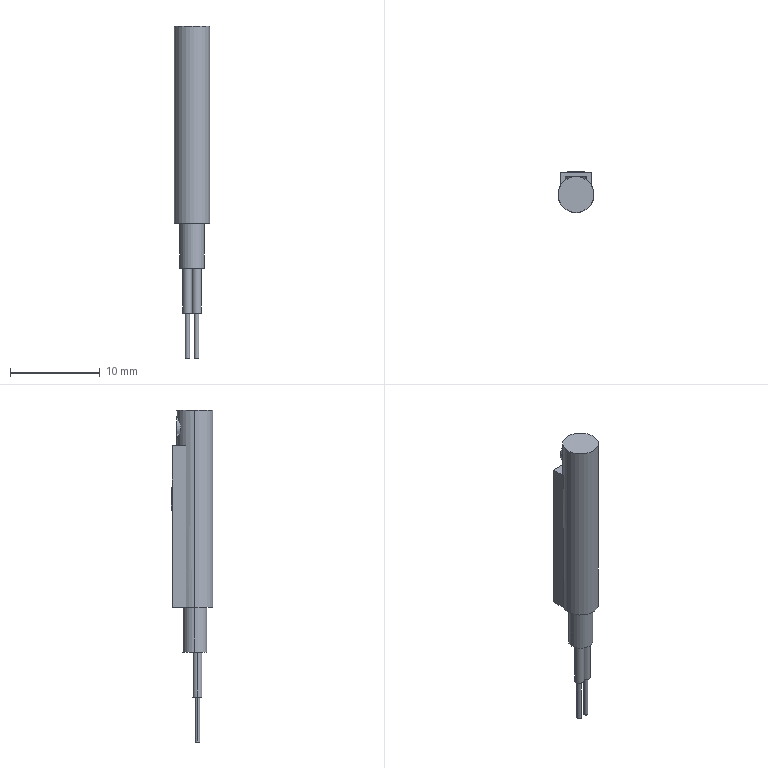Part | NX | 1 solid | 38 faces | box 4 x 4.6 x 37 mm | volume 364.626 mm3 | plane 21 | cylinder 17 | commonest cylinder face diameters 0.5 x4 1 x4 2.4 x3 2.5 x2 2.7 x2 4 x2
STEP:
#1=CARTESIAN_POINT('',(0.,2.,-3.2));
#2=VERTEX_POINT('',#1);
#3=CARTESIAN_POINT('',(0.,1.,-3.2));
#4=VERTEX_POINT('',#3);
#5=CARTESIAN_POINT('',(0.,2.,-3.2));
#6=DIRECTION('',(0.,-1.,0.));
#7=VECTOR('',#6,1000.);
#8=LINE('',#5,#7);
#9=EDGE_CURVE('',#2,#4,#8,.T.);
#10=ORIENTED_EDGE('',*,*,#9,.F.);
#11=CARTESIAN_POINT('',(1.007,2.,-1.347));
#12=VERTEX_POINT('',#11);
#13=CARTESIAN_POINT('',(0.,2.,-2.));
#14=DIRECTION('',(0.,1.,0.));
#15=DIRECTION('',(0.,0.,1.));
#16=AXIS2_PLACEMENT_3D('',#13,#14,#15);
#17=CIRCLE('',#16,1.2);
#18=EDGE_CURVE('',#12,#2,#17,.T.);
#19=ORIENTED_EDGE('',*,*,#18,.F.);
#20=CARTESIAN_POINT('',(1.007,1.,-1.347));
#21=VERTEX_POINT('',#20);
#22=CARTESIAN_POINT('',(1.007,1.,-1.347));
#23=DIRECTION('',(0.,1.,0.));
#24=VECTOR('',#23,1000.);
#25=LINE('',#22,#24);
#26=EDGE_CURVE('',#21,#12,#25,.T.);
#27=ORIENTED_EDGE('',*,*,#26,.F.);
#28=CARTESIAN_POINT('',(0.,1.,-2.));
#29=DIRECTION('',(0.,1.,0.));
#30=DIRECTION('',(0.,0.,1.));
#31=AXIS2_PLACEMENT_3D('',#28,#29,#30);
#32=CIRCLE('',#31,1.2);
#33=EDGE_CURVE('',#21,#4,#32,.T.);
#34=ORIENTED_EDGE('',*,*,#33,.T.);
#35=EDGE_LOOP('',(#10,#19,#27,#34));
#36=FACE_BOUND('',#35,.T.);
#37=CARTESIAN_POINT('',(0.,2.,-2.));
#38=DIRECTION('',(0.,-1.,0.));
#39=DIRECTION('',(0.,0.,-1.));
#40=AXIS2_PLACEMENT_3D('',#37,#38,#39);
#41=CYLINDRICAL_SURFACE('',#40,1.2);
#42=ADVANCED_FACE('',(#36),#41,.T.);
#43=CARTESIAN_POINT('',(0.,2.,-0.75));
#44=VERTEX_POINT('',#43);
#45=CARTESIAN_POINT('',(0.,2.,-3.25));
#46=VERTEX_POINT('',#45);
#47=CARTESIAN_POINT('',(0.,2.,-0.75));
#48=CARTESIAN_POINT('',(0.02817,2.,-0.75));
#49=CARTESIAN_POINT('',(0.05639,1.999,-0.751));
#50=CARTESIAN_POINT('',(0.08452,1.998,-0.7529));
#51=CARTESIAN_POINT('',(0.1126,1.997,-0.7548));
#52=CARTESIAN_POINT('',(0.1407,1.995,-0.7576));
#53=CARTESIAN_POINT('',(0.1685,1.993,-0.7614));
#54=CARTESIAN_POINT('',(0.1824,1.992,-0.7633));
#55=CARTESIAN_POINT('',(0.1963,1.99,-0.7654));
#56=CARTESIAN_POINT('',(0.2101,1.989,-0.7678));
#57=CARTESIAN_POINT('',(0.2238,1.987,-0.7701));
#58=CARTESIAN_POINT('',(0.2376,1.986,-0.7727));
#59=CARTESIAN_POINT('',(0.2513,1.984,-0.7755));
#60=CARTESIAN_POINT('',(0.2787,1.981,-0.7811));
#61=CARTESIAN_POINT('',(0.3059,1.977,-0.7877));
#62=CARTESIAN_POINT('',(0.3327,1.972,-0.7951));
#63=CARTESIAN_POINT('',(0.3596,1.968,-0.8025));
#64=CARTESIAN_POINT('',(0.3861,1.963,-0.8108));
#65=CARTESIAN_POINT('',(0.4122,1.957,-0.8199));
#66=CARTESIAN_POINT('',(0.4383,1.952,-0.829));
#67=CARTESIAN_POINT('',(0.464,1.946,-0.839));
#68=CARTESIAN_POINT('',(0.4892,1.939,-0.8497));
#69=CARTESIAN_POINT('',(0.5144,1.933,-0.8604));
#70=CARTESIAN_POINT('',(0.5393,1.926,-0.872));
#71=CARTESIAN_POINT('',(0.5637,1.919,-0.8843));
#72=CARTESIAN_POINT('',(0.5881,1.912,-0.8966));
#73=CARTESIAN_POINT('',(0.612,1.904,-0.9097));
#74=CARTESIAN_POINT('',(0.6354,1.896,-0.9235));
#75=CARTESIAN_POINT('',(0.6588,1.889,-0.9373));
#76=CARTESIAN_POINT('',(0.6817,1.88,-0.9519));
#77=CARTESIAN_POINT('',(0.704,1.872,-0.9671));
#78=CARTESIAN_POINT('',(0.7263,1.864,-0.9823));
#79=CARTESIAN_POINT('',(0.748,1.855,-0.9981));
#80=CARTESIAN_POINT('',(0.7691,1.846,-1.015));
#81=CARTESIAN_POINT('',(0.7901,1.837,-1.031));
#82=CARTESIAN_POINT('',(0.8106,1.828,-1.048));
#83=CARTESIAN_POINT('',(0.8306,1.819,-1.066));
#84=CARTESIAN_POINT('',(0.8506,1.81,-1.084));
#85=CARTESIAN_POINT('',(0.87,1.801,-1.102));
#86=CARTESIAN_POINT('',(0.8888,1.792,-1.121));
#87=CARTESIAN_POINT('',(0.9076,1.782,-1.14));
#88=CARTESIAN_POINT('',(0.9258,1.773,-1.16));
#89=CARTESIAN_POINT('',(0.9434,1.764,-1.18));
#90=CARTESIAN_POINT('',(0.961,1.754,-1.2));
#91=CARTESIAN_POINT('',(0.9779,1.745,-1.221));
#92=CARTESIAN_POINT('',(0.9942,1.735,-1.242));
#93=CARTESIAN_POINT('',(1.01,1.726,-1.264));
#94=CARTESIAN_POINT('',(1.026,1.717,-1.285));
#95=CARTESIAN_POINT('',(1.041,1.708,-1.308));
#96=CARTESIAN_POINT('',(1.056,1.699,-1.33));
#97=CARTESIAN_POINT('',(1.07,1.69,-1.353));
#98=CARTESIAN_POINT('',(1.083,1.681,-1.376));
#99=CARTESIAN_POINT('',(1.09,1.677,-1.388));
#100=CARTESIAN_POINT('',(1.096,1.673,-1.399));
#101=CARTESIAN_POINT('',(1.102,1.669,-1.411));
#102=CARTESIAN_POINT('',(1.109,1.665,-1.422));
#103=CARTESIAN_POINT('',(1.115,1.661,-1.434));
#104=CARTESIAN_POINT('',(1.121,1.657,-1.446));
#105=CARTESIAN_POINT('',(1.132,1.649,-1.47));
#106=CARTESIAN_POINT('',(1.143,1.641,-1.494));
#107=CARTESIAN_POINT('',(1.154,1.634,-1.519));
#108=CARTESIAN_POINT('',(1.164,1.626,-1.544));
#109=CARTESIAN_POINT('',(1.174,1.619,-1.569));
#110=CARTESIAN_POINT('',(1.182,1.613,-1.595));
#111=CARTESIAN_POINT('',(1.191,1.607,-1.62));
#112=CARTESIAN_POINT('',(1.199,1.601,-1.646));
#113=CARTESIAN_POINT('',(1.206,1.595,-1.673));
#114=CARTESIAN_POINT('',(1.214,1.59,-1.699));
#115=CARTESIAN_POINT('',(1.22,1.585,-1.726));
#116=CARTESIAN_POINT('',(1.225,1.581,-1.753));
#117=CARTESIAN_POINT('',(1.231,1.577,-1.779));
#118=CARTESIAN_POINT('',(1.235,1.573,-1.806));
#119=CARTESIAN_POINT('',(1.239,1.57,-1.834));
#120=CARTESIAN_POINT('',(1.243,1.567,-1.861));
#121=CARTESIAN_POINT('',(1.245,1.565,-1.888));
#122=CARTESIAN_POINT('',(1.247,1.563,-1.916));
#123=CARTESIAN_POINT('',(1.248,1.563,-1.93));
#124=CARTESIAN_POINT('',(1.249,1.562,-1.944));
#125=CARTESIAN_POINT('',(1.249,1.562,-1.958));
#126=CARTESIAN_POINT('',(1.25,1.561,-1.972));
#127=CARTESIAN_POINT('',(1.25,1.561,-1.986));
#128=CARTESIAN_POINT('',(1.25,1.561,-2.));
#129=CARTESIAN_POINT('',(1.25,1.561,-2.014));
#130=CARTESIAN_POINT('',(1.25,1.561,-2.028));
#131=CARTESIAN_POINT('',(1.249,1.562,-2.042));
#132=CARTESIAN_POINT('',(1.249,1.562,-2.055));
#133=CARTESIAN_POINT('',(1.248,1.563,-2.069));
#134=CARTESIAN_POINT('',(1.247,1.563,-2.083));
#135=CARTESIAN_POINT('',(1.245,1.565,-2.111));
#136=CARTESIAN_POINT('',(1.243,1.567,-2.139));
#137=CARTESIAN_POINT('',(1.239,1.57,-2.166));
#138=CARTESIAN_POINT('',(1.237,1.571,-2.18));
#139=CARTESIAN_POINT('',(1.235,1.573,-2.193));
#140=CARTESIAN_POINT('',(1.233,1.575,-2.207));
#141=CARTESIAN_POINT('',(1.231,1.577,-2.22));
#142=CARTESIAN_POINT('',(1.228,1.579,-2.234));
#143=CARTESIAN_POINT('',(1.225,1.581,-2.247));
#144=CARTESIAN_POINT('',(1.22,1.585,-2.274));
#145=CARTESIAN_POINT('',(1.214,1.59,-2.3));
#146=CARTESIAN_POINT('',(1.207,1.595,-2.327));
#147=CARTESIAN_POINT('',(1.199,1.6,-2.353));
#148=CARTESIAN_POINT('',(1.191,1.606,-2.379));
#149=CARTESIAN_POINT('',(1.183,1.613,-2.405));
#150=CARTESIAN_POINT('',(1.174,1.619,-2.43));
#151=CARTESIAN_POINT('',(1.164,1.626,-2.456));
#152=CARTESIAN_POINT('',(1.154,1.633,-2.48));
#153=CARTESIAN_POINT('',(1.144,1.641,-2.505));
#154=CARTESIAN_POINT('',(1.133,1.648,-2.529));
#155=CARTESIAN_POINT('',(1.121,1.656,-2.553));
#156=CARTESIAN_POINT('',(1.115,1.66,-2.565));
#157=CARTESIAN_POINT('',(1.109,1.664,-2.577));
#158=CARTESIAN_POINT('',(1.103,1.668,-2.589));
#159=CARTESIAN_POINT('',(1.097,1.673,-2.6));
#160=CARTESIAN_POINT('',(1.09,1.677,-2.612));
#161=CARTESIAN_POINT('',(1.084,1.681,-2.623));
#162=CARTESIAN_POINT('',(1.07,1.69,-2.646));
#163=CARTESIAN_POINT('',(1.056,1.699,-2.669));
#164=CARTESIAN_POINT('',(1.041,1.708,-2.692));
#165=CARTESIAN_POINT('',(1.026,1.717,-2.714));
#166=CARTESIAN_POINT('',(1.011,1.726,-2.736));
#167=CARTESIAN_POINT('',(0.9946,1.735,-2.757));
#168=CARTESIAN_POINT('',(0.9784,1.744,-2.778));
#169=CARTESIAN_POINT('',(0.9615,1.754,-2.799));
#170=CARTESIAN_POINT('',(0.9439,1.763,-2.819));
#171=CARTESIAN_POINT('',(0.9264,1.773,-2.84));
#172=CARTESIAN_POINT('',(0.9082,1.782,-2.859));
#173=CARTESIAN_POINT('',(0.8894,1.791,-2.878));
#174=CARTESIAN_POINT('',(0.8706,1.801,-2.897));
#175=CARTESIAN_POINT('',(0.8512,1.81,-2.916));
#176=CARTESIAN_POINT('',(0.8313,1.819,-2.933));
#177=CARTESIAN_POINT('',(0.8213,1.824,-2.942));
#178=CARTESIAN_POINT('',(0.8112,1.828,-2.951));
#179=CARTESIAN_POINT('',(0.801,1.833,-2.96));
#180=CARTESIAN_POINT('',(0.7908,1.837,-2.968));
#181=CARTESIAN_POINT('',(0.7804,1.842,-2.977));
#182=CARTESIAN_POINT('',(0.7698,1.846,-2.985));
#183=CARTESIAN_POINT('',(0.7487,1.855,-3.001));
#184=CARTESIAN_POINT('',(0.727,1.863,-3.017));
#185=CARTESIAN_POINT('',(0.7046,1.872,-3.032));
#186=CARTESIAN_POINT('',(0.6823,1.88,-3.048));
#187=CARTESIAN_POINT('',(0.6594,1.888,-3.062));
#188=CARTESIAN_POINT('',(0.6359,1.896,-3.076));
#189=CARTESIAN_POINT('',(0.6124,1.904,-3.09));
#190=CARTESIAN_POINT('',(0.5885,1.912,-3.103));
#191=CARTESIAN_POINT('',(0.564,1.919,-3.116));
#192=CARTESIAN_POINT('',(0.5395,1.926,-3.128));
#193=CARTESIAN_POINT('',(0.5146,1.933,-3.139));
#194=CARTESIAN_POINT('',(0.4893,1.939,-3.15));
#195=CARTESIAN_POINT('',(0.464,1.946,-3.161));
#196=CARTESIAN_POINT('',(0.4383,1.952,-3.171));
#197=CARTESIAN_POINT('',(0.4122,1.957,-3.18));
#198=CARTESIAN_POINT('',(0.3862,1.963,-3.189));
#199=CARTESIAN_POINT('',(0.3597,1.968,-3.197));
#200=CARTESIAN_POINT('',(0.3328,1.972,-3.205));
#201=CARTESIAN_POINT('',(0.306,1.977,-3.212));
#202=CARTESIAN_POINT('',(0.2788,1.981,-3.219));
#203=CARTESIAN_POINT('',(0.2513,1.984,-3.224));
#204=CARTESIAN_POINT('',(0.2239,1.988,-3.23));
#205=CARTESIAN_POINT('',(0.1962,1.991,-3.235));
#206=CARTESIAN_POINT('',(0.1684,1.993,-3.239));
#207=CARTESIAN_POINT('',(0.1406,1.995,-3.242));
#208=CARTESIAN_POINT('',(0.1127,1.997,-3.245));
#209=CARTESIAN_POINT('',(0.08455,1.998,-3.247));
#210=CARTESIAN_POINT('',(0.05645,1.999,-3.249));
#211=CARTESIAN_POINT('',(0.02822,2.,-3.25));
#212=CARTESIAN_POINT('',(0.,2.,-3.25));
#213=B_SPLINE_CURVE_WITH_KNOTS('',3,(#47,#48,#49,#50,#51,#52,#53,#54,#55,#56,#57,#58,#59,#60,#61,#62,#63,#64,#65,#66,#67,#68,#69,#70,#71,#72,#73,#74,#75,#76,#77,#78,#79,#80,#81,#82,#83,#84,#85,#86,#87,#88,#89,#90,#91,#92,#93,#94,#95,#96,#97,#98,#99,#100,#101,#102,#103,#104,#105,#106,#107,#108,#109,#110,#111,#112,#113,#114,#115,#116,#117,#118,#119,#120,#121,#122,#123,#124,#125,#126,#127,#128,#129,#130,#131,#132,#133,#134,#135,#136,#137,#138,#139,#140,#141,#142,#143,#144,#145,#146,#147,#148,#149,#150,#151,#152,#153,#154,#155,#156,#157,#158,#159,#160,#161,#162,#163,#164,#165,#166,#167,#168,#169,#170,#171,#172,#173,#174,#175,#176,#177,#178,#179,#180,#181,#182,#183,#184,#185,#186,#187,#188,#189,#190,#191,#192,#193,#194,#195,#196,#197,#198,#199,#200,#201,#202,#203,#204,#205,#206,#207,#208,#209,#210,#211,#212),.UNSPECIFIED.,.F.,.F.,(4,3,3,3,3,3,3,3,3,3,3,3,3,3,3,3,3,3,3,3,3,3,3,3,3,3,3,3,3,3,3,3,3,3,3,3,3,3,3,3,3,3,3,3,3,3,3,3,3,3,3,3,3,3,3,4),(0.,0.08461,0.1692,0.2114,0.2537,0.3383,0.4229,0.5074,0.592,0.6768,0.7617,0.8463,0.9308,1.016,1.101,1.186,1.271,1.356,1.397,1.439,1.522,1.606,1.689,1.773,1.856,1.939,1.981,2.022,2.064,2.106,2.189,2.231,2.272,2.356,2.439,2.522,2.606,2.647,2.689,2.774,2.859,2.944,3.029,3.113,3.156,3.198,3.283,3.368,3.453,3.538,3.622,3.707,3.792,3.876,3.961,4.045),.UNSPECIFIED.);
#214=EDGE_CURVE('',#44,#46,#213,.T.);
#215=ORIENTED_EDGE('',*,*,#214,.T.);
#216=CARTESIAN_POINT('',(0.,1.,-3.25));
#217=VERTEX_POINT('',#216);
#218=CARTESIAN_POINT('',(0.,2.6,-3.25));
#219=DIRECTION('',(0.,-1.,0.));
#220=VECTOR('',#219,1000.);
#221=LINE('',#218,#220);
#222=EDGE_CURVE('',#217,#46,#221,.F.);
#223=ORIENTED_EDGE('',*,*,#222,.F.);
#224=CARTESIAN_POINT('',(0.,1.,-0.75));
#225=VERTEX_POINT('',#224);
#226=CARTESIAN_POINT('',(0.,1.,-2.));
#227=DIRECTION('',(0.,1.,0.));
#228=DIRECTION('',(0.,0.,1.));
#229=AXIS2_PLACEMENT_3D('',#226,#227,#228);
#230=CIRCLE('',#229,1.25);
#231=EDGE_CURVE('',#225,#217,#230,.T.);
#232=ORIENTED_EDGE('',*,*,#231,.F.);
#233=CARTESIAN_POINT('',(0.,2.6,-0.75));
#234=DIRECTION('',(0.,-1.,0.));
#235=VECTOR('',#234,1000.);
#236=LINE('',#233,#235);
#237=EDGE_CURVE('',#225,#44,#236,.F.);
#238=ORIENTED_EDGE('',*,*,#237,.T.);
#239=EDGE_LOOP('',(#215,#223,#232,#238));
#240=FACE_BOUND('',#239,.T.);
#241=CARTESIAN_POINT('',(0.,2.6,-2.));
#242=DIRECTION('',(0.,-1.,0.));
#243=DIRECTION('',(0.,0.,-1.));
#244=AXIS2_PLACEMENT_3D('',#241,#242,#243);
#245=CYLINDRICAL_SURFACE('',#244,1.25);
#246=ADVANCED_FACE('',(#240),#245,.F.);
#247=CARTESIAN_POINT('',(-0.7696,-0.3,-32.));
#248=VERTEX_POINT('',#247);
#249=CARTESIAN_POINT('',(-0.2696,-0.3,-32.));
#250=VERTEX_POINT('',#249);
#251=CARTESIAN_POINT('',(-0.5196,-0.3,-32.));
#252=DIRECTION('',(0.,0.,-1.));
#253=DIRECTION('',(1.,0.,0.));
#254=AXIS2_PLACEMENT_3D('',#251,#252,#253);
#255=CIRCLE('',#254,0.25);
#256=EDGE_CURVE('',#248,#250,#255,.T.);
#257=ORIENTED_EDGE('',*,*,#256,.T.);
#258=CARTESIAN_POINT('',(-0.2696,-0.3,-37.));
#259=VERTEX_POINT('',#258);
#260=CARTESIAN_POINT('',(-0.2696,-0.3,-37.));
#261=DIRECTION('',(0.,0.,1.));
#262=VECTOR('',#261,1000.);
#263=LINE('',#260,#262);
#264=EDGE_CURVE('',#259,#250,#263,.T.);
#265=ORIENTED_EDGE('',*,*,#264,.F.);
#266=CARTESIAN_POINT('',(-0.7696,-0.3,-37.));
#267=VERTEX_POINT('',#266);
#268=CARTESIAN_POINT('',(-0.5196,-0.3,-37.));
#269=DIRECTION('',(0.,0.,-1.));
#270=DIRECTION('',(1.,0.,0.));
#271=AXIS2_PLACEMENT_3D('',#268,#269,#270);
#272=CIRCLE('',#271,0.25);
#273=EDGE_CURVE('',#267,#259,#272,.T.);
#274=ORIENTED_EDGE('',*,*,#273,.F.);
#275=CARTESIAN_POINT('',(-0.7696,-0.3,-37.));
#276=DIRECTION('',(0.,0.,1.));
#277=VECTOR('',#276,1000.);
#278=LINE('',#275,#277);
#279=EDGE_CURVE('',#267,#248,#278,.T.);
#280=ORIENTED_EDGE('',*,*,#279,.T.);
#281=EDGE_LOOP('',(#257,#265,#274,#280));
#282=FACE_BOUND('',#281,.T.);
#283=CARTESIAN_POINT('',(-0.5196,-0.3,-37.));
#284=DIRECTION('',(0.,0.,1.));
#285=DIRECTION('',(1.,0.,0.));
#286=AXIS2_PLACEMENT_3D('',#283,#284,#285);
#287=CYLINDRICAL_SURFACE('',#286,0.25);
#288=ADVANCED_FACE('',(#282),#287,.T.);
#289=CARTESIAN_POINT('',(0.7696,-0.3,-32.));
#290=VERTEX_POINT('',#289);
#291=CARTESIAN_POINT('',(0.2696,-0.3,-32.));
#292=VERTEX_POINT('',#291);
#293=CARTESIAN_POINT('',(0.5196,-0.3,-32.));
#294=DIRECTION('',(0.,0.,-1.));
#295=DIRECTION('',(-1.,0.,0.));
#296=AXIS2_PLACEMENT_3D('',#293,#294,#295);
#297=CIRCLE('',#296,0.25);
#298=EDGE_CURVE('',#290,#292,#297,.T.);
#299=ORIENTED_EDGE('',*,*,#298,.T.);
#300=CARTESIAN_POINT('',(0.2696,-0.3,-37.));
#301=VERTEX_POINT('',#300);
#302=CARTESIAN_POINT('',(0.2696,-0.3,-37.));
#303=DIRECTION('',(0.,0.,1.));
#304=VECTOR('',#303,1000.);
#305=LINE('',#302,#304);
#306=EDGE_CURVE('',#292,#301,#305,.F.);
#307=ORIENTED_EDGE('',*,*,#306,.T.);
#308=CARTESIAN_POINT('',(0.7696,-0.3,-37.));
#309=VERTEX_POINT('',#308);
#310=CARTESIAN_POINT('',(0.5196,-0.3,-37.));
#311=DIRECTION('',(0.,0.,-1.));
#312=DIRECTION('',(-1.,0.,0.));
#313=AXIS2_PLACEMENT_3D('',#310,#311,#312);
#314=CIRCLE('',#313,0.25);
#315=EDGE_CURVE('',#309,#301,#314,.T.);
#316=ORIENTED_EDGE('',*,*,#315,.F.);
#317=CARTESIAN_POINT('',(0.7696,-0.3,-37.));
#318=DIRECTION('',(0.,0.,1.));
#319=VECTOR('',#318,1000.);
#320=LINE('',#317,#319);
#321=EDGE_CURVE('',#290,#309,#320,.F.);
#322=ORIENTED_EDGE('',*,*,#321,.F.);
#323=EDGE_LOOP('',(#299,#307,#316,#322));
#324=FACE_BOUND('',#323,.T.);
#325=CARTESIAN_POINT('',(0.5196,-0.3,-37.));
#326=DIRECTION('',(0.,0.,1.));
#327=DIRECTION('',(1.,0.,0.));
#328=AXIS2_PLACEMENT_3D('',#325,#326,#327);
#329=CYLINDRICAL_SURFACE('',#328,0.25);
#330=ADVANCED_FACE('',(#324),#329,.T.);
#331=CARTESIAN_POINT('',(-1.02,-0.3,-27.));
#332=VERTEX_POINT('',#331);
#333=CARTESIAN_POINT('',(-0.01962,-0.3,-27.));
#334=VERTEX_POINT('',#333);
#335=CARTESIAN_POINT('',(-0.5196,-0.3,-27.));
#336=DIRECTION('',(0.,0.,-1.));
#337=DIRECTION('',(-1.,0.,0.));
#338=AXIS2_PLACEMENT_3D('',#335,#336,#337);
#339=CIRCLE('',#338,0.5);
#340=EDGE_CURVE('',#332,#334,#339,.T.);
#341=ORIENTED_EDGE('',*,*,#340,.T.);
#342=CARTESIAN_POINT('',(-0.01962,-0.3,-32.));
#343=VERTEX_POINT('',#342);
#344=CARTESIAN_POINT('',(-0.01962,-0.3,-32.));
#345=DIRECTION('',(0.,0.,1.));
#346=VECTOR('',#345,1000.);
#347=LINE('',#344,#346);
#348=EDGE_CURVE('',#343,#334,#347,.T.);
#349=ORIENTED_EDGE('',*,*,#348,.F.);
#350=CARTESIAN_POINT('',(-1.02,-0.3,-32.));
#351=VERTEX_POINT('',#350);
#352=CARTESIAN_POINT('',(-0.5196,-0.3,-32.));
#353=DIRECTION('',(0.,0.,-1.));
#354=DIRECTION('',(-1.,0.,0.));
#355=AXIS2_PLACEMENT_3D('',#352,#353,#354);
#356=CIRCLE('',#355,0.5);
#357=EDGE_CURVE('',#351,#343,#356,.T.);
#358=ORIENTED_EDGE('',*,*,#357,.F.);
#359=CARTESIAN_POINT('',(-1.02,-0.3,-32.));
#360=DIRECTION('',(0.,0.,1.));
#361=VECTOR('',#360,1000.);
#362=LINE('',#359,#361);
#363=EDGE_CURVE('',#351,#332,#362,.T.);
#364=ORIENTED_EDGE('',*,*,#363,.T.);
#365=EDGE_LOOP('',(#341,#349,#358,#364));
#366=FACE_BOUND('',#365,.T.);
#367=CARTESIAN_POINT('',(-0.5196,-0.3,-32.));
#368=DIRECTION('',(0.,0.,1.));
#369=DIRECTION('',(1.,0.,0.));
#370=AXIS2_PLACEMENT_3D('',#367,#368,#369);
#371=CYLINDRICAL_SURFACE('',#370,0.5);
#372=ADVANCED_FACE('',(#366),#371,.T.);
#373=CARTESIAN_POINT('',(1.02,-0.3,-27.));
#374=VERTEX_POINT('',#373);
#375=CARTESIAN_POINT('',(0.01962,-0.3,-27.));
#376=VERTEX_POINT('',#375);
#377=CARTESIAN_POINT('',(0.5196,-0.3,-27.));
#378=DIRECTION('',(0.,0.,-1.));
#379=DIRECTION('',(-1.,0.,0.));
#380=AXIS2_PLACEMENT_3D('',#377,#378,#379);
#381=CIRCLE('',#380,0.5);
#382=EDGE_CURVE('',#374,#376,#381,.T.);
#383=ORIENTED_EDGE('',*,*,#382,.T.);
#384=CARTESIAN_POINT('',(0.01962,-0.3,-32.));
#385=VERTEX_POINT('',#384);
#386=CARTESIAN_POINT('',(0.01962,-0.3,-32.));
#387=DIRECTION('',(0.,0.,1.));
#388=VECTOR('',#387,1000.);
#389=LINE('',#386,#388);
#390=EDGE_CURVE('',#376,#385,#389,.F.);
#391=ORIENTED_EDGE('',*,*,#390,.T.);
#392=CARTESIAN_POINT('',(1.02,-0.3,-32.));
#393=VERTEX_POINT('',#392);
#394=CARTESIAN_POINT('',(0.5196,-0.3,-32.));
#395=DIRECTION('',(0.,0.,-1.));
#396=DIRECTION('',(-1.,0.,0.));
#397=AXIS2_PLACEMENT_3D('',#394,#395,#396);
#398=CIRCLE('',#397,0.5);
#399=EDGE_CURVE('',#393,#385,#398,.T.);
#400=ORIENTED_EDGE('',*,*,#399,.F.);
#401=CARTESIAN_POINT('',(1.02,-0.3,-32.));
#402=DIRECTION('',(0.,0.,1.));
#403=VECTOR('',#402,1000.);
#404=LINE('',#401,#403);
#405=EDGE_CURVE('',#374,#393,#404,.F.);
#406=ORIENTED_EDGE('',*,*,#405,.F.);
#407=EDGE_LOOP('',(#383,#391,#400,#406));
#408=FACE_BOUND('',#407,.T.);
#409=CARTESIAN_POINT('',(0.5196,-0.3,-32.));
#410=DIRECTION('',(0.,0.,1.));
#411=DIRECTION('',(1.,0.,0.));
#412=AXIS2_PLACEMENT_3D('',#409,#410,#411);
#413=CYLINDRICAL_SURFACE('',#412,0.5);
#414=ADVANCED_FACE('',(#408),#413,.T.);
#415=CARTESIAN_POINT('',(1.35,0.,-27.));
#416=VERTEX_POINT('',#415);
#417=CARTESIAN_POINT('',(-1.35,0.,-27.));
#418=VERTEX_POINT('',#417);
#419=CARTESIAN_POINT('',(0.,0.,-27.));
#420=DIRECTION('',(0.,0.,-1.));
#421=DIRECTION('',(-1.,0.,0.));
#422=AXIS2_PLACEMENT_3D('',#419,#420,#421);
#423=CIRCLE('',#422,1.35);
#424=EDGE_CURVE('',#416,#418,#423,.T.);
#425=ORIENTED_EDGE('',*,*,#424,.F.);
#426=CARTESIAN_POINT('',(1.35,0.,-22.));
#427=VERTEX_POINT('',#426);
#428=CARTESIAN_POINT('',(1.35,0.,-27.));
#429=DIRECTION('',(0.,0.,1.));
#430=VECTOR('',#429,1000.);
#431=LINE('',#428,#430);
#432=EDGE_CURVE('',#416,#427,#431,.T.);
#433=ORIENTED_EDGE('',*,*,#432,.T.);
#434=CARTESIAN_POINT('',(-1.35,0.,-22.));
#435=VERTEX_POINT('',#434);
#436=CARTESIAN_POINT('',(0.,0.,-22.));
#437=DIRECTION('',(0.,0.,-1.));
#438=DIRECTION('',(1.,0.,0.));
#439=AXIS2_PLACEMENT_3D('',#436,#437,#438);
#440=CIRCLE('',#439,1.35);
#441=EDGE_CURVE('',#427,#435,#440,.T.);
#442=ORIENTED_EDGE('',*,*,#441,.T.);
#443=CARTESIAN_POINT('',(-1.35,0.,-27.));
#444=DIRECTION('',(0.,0.,1.));
#445=VECTOR('',#444,1000.);
#446=LINE('',#443,#445);
#447=EDGE_CURVE('',#418,#435,#446,.T.);
#448=ORIENTED_EDGE('',*,*,#447,.F.);
#449=EDGE_LOOP('',(#425,#433,#442,#448));
#450=FACE_BOUND('',#449,.T.);
#451=CARTESIAN_POINT('',(0.,0.,-27.));
#452=DIRECTION('',(0.,0.,1.));
#453=DIRECTION('',(1.,0.,0.));
#454=AXIS2_PLACEMENT_3D('',#451,#452,#453);
#455=CYLINDRICAL_SURFACE('',#454,1.35);
#456=ADVANCED_FACE('',(#450),#455,.T.);
#457=CARTESIAN_POINT('',(-2.,0.,0.));
#458=VERTEX_POINT('',#457);
#459=CARTESIAN_POINT('',(2.,0.,0.));
#460=VERTEX_POINT('',#459);
#461=CARTESIAN_POINT('',(0.,0.,0.));
#462=DIRECTION('',(0.,0.,1.));
#463=DIRECTION('',(1.,0.,0.));
#464=AXIS2_PLACEMENT_3D('',#461,#462,#463);
#465=CIRCLE('',#464,2.);
#466=EDGE_CURVE('',#458,#460,#465,.T.);
#467=ORIENTED_EDGE('',*,*,#466,.F.);
#468=CARTESIAN_POINT('',(-2.,0.,-22.));
#469=VERTEX_POINT('',#468);
#470=CARTESIAN_POINT('',(-2.,0.,-22.));
#471=DIRECTION('',(0.,0.,1.));
#472=VECTOR('',#471,1000.);
#473=LINE('',#470,#472);
#474=EDGE_CURVE('',#458,#469,#473,.F.);
#475=ORIENTED_EDGE('',*,*,#474,.T.);
#476=CARTESIAN_POINT('',(2.,0.,-22.));
#477=VERTEX_POINT('',#476);
#478=CARTESIAN_POINT('',(0.,0.,-22.));
#479=DIRECTION('',(0.,0.,1.));
#480=DIRECTION('',(1.,0.,0.));
#481=AXIS2_PLACEMENT_3D('',#478,#479,#480);
#482=CIRCLE('',#481,2.);
#483=EDGE_CURVE('',#469,#477,#482,.T.);
#484=ORIENTED_EDGE('',*,*,#483,.T.);
#485=CARTESIAN_POINT('',(2.,0.,-22.));
#486=DIRECTION('',(0.,0.,1.));
#487=VECTOR('',#486,1000.);
#488=LINE('',#485,#487);
#489=EDGE_CURVE('',#460,#477,#488,.F.);
#490=ORIENTED_EDGE('',*,*,#489,.F.);
#491=EDGE_LOOP('',(#467,#475,#484,#490));
#492=FACE_BOUND('',#491,.T.);
#493=CARTESIAN_POINT('',(0.,0.,-22.));
#494=DIRECTION('',(0.,0.,1.));
#495=DIRECTION('',(1.,0.,0.));
#496=AXIS2_PLACEMENT_3D('',#493,#494,#495);
#497=CYLINDRICAL_SURFACE('',#496,2.);
#498=ADVANCED_FACE('',(#492),#497,.T.);
#499=CARTESIAN_POINT('',(-1.007,2.,-2.653));
#500=VERTEX_POINT('',#499);
#501=CARTESIAN_POINT('',(0.6531,2.,-0.9933));
#502=VERTEX_POINT('',#501);
#503=CARTESIAN_POINT('',(0.,2.,-2.));
#504=DIRECTION('',(0.,1.,0.));
#505=DIRECTION('',(0.,0.,1.));
#506=AXIS2_PLACEMENT_3D('',#503,#504,#505);
#507=CIRCLE('',#506,1.2);
#508=EDGE_CURVE('',#500,#502,#507,.T.);
#509=ORIENTED_EDGE('',*,*,#508,.F.);
#510=CARTESIAN_POINT('',(-1.007,1.,-2.653));
#511=VERTEX_POINT('',#510);
#512=CARTESIAN_POINT('',(-1.007,1.,-2.653));
#513=DIRECTION('',(0.,1.,0.));
#514=VECTOR('',#513,1000.);
#515=LINE('',#512,#514);
#516=EDGE_CURVE('',#511,#500,#515,.T.);
#517=ORIENTED_EDGE('',*,*,#516,.F.);
#518=CARTESIAN_POINT('',(0.6531,1.,-0.9933));
#519=VERTEX_POINT('',#518);
#520=CARTESIAN_POINT('',(0.,1.,-2.));
#521=DIRECTION('',(0.,1.,0.));
#522=DIRECTION('',(0.,0.,1.));
#523=AXIS2_PLACEMENT_3D('',#520,#521,#522);
#524=CIRCLE('',#523,1.2);
#525=EDGE_CURVE('',#511,#519,#524,.T.);
#526=ORIENTED_EDGE('',*,*,#525,.T.);
#527=CARTESIAN_POINT('',(0.6531,1.,-0.9933));
#528=DIRECTION('',(0.,1.,0.));
#529=VECTOR('',#528,1000.);
#530=LINE('',#527,#529);
#531=EDGE_CURVE('',#519,#502,#530,.T.);
#532=ORIENTED_EDGE('',*,*,#531,.T.);
#533=EDGE_LOOP('',(#509,#517,#526,#532));
#534=FACE_BOUND('',#533,.T.);
#535=CARTESIAN_POINT('',(0.,2.,-2.));
#536=DIRECTION('',(0.,-1.,0.));
#537=DIRECTION('',(0.,0.,-1.));
#538=AXIS2_PLACEMENT_3D('',#535,#536,#537);
#539=CYLINDRICAL_SURFACE('',#538,1.2);
#540=ADVANCED_FACE('',(#534),#539,.T.);
#541=CARTESIAN_POINT('',(0.6531,2.,-0.9933));
#542=DIRECTION('',(0.7071,0.,0.7071));
#543=VECTOR('',#542,1000.);
#544=LINE('',#541,#543);
#545=EDGE_CURVE('',#500,#502,#544,.T.);
#546=ORIENTED_EDGE('',*,*,#545,.F.);
#547=ORIENTED_EDGE('',*,*,#508,.T.);
#548=EDGE_LOOP('',(#546,#547));
#549=FACE_BOUND('',#548,.T.);
#550=CARTESIAN_POINT('',(0.,2.,-2.));
#551=DIRECTION('',(0.,1.,0.));
#552=DIRECTION('',(1.,0.,0.));
#553=AXIS2_PLACEMENT_3D('',#550,#551,#552);
#554=PLANE('',#553);
#555=ADVANCED_FACE('',(#549),#554,.T.);
#556=CARTESIAN_POINT('',(0.,1.,-2.));
#557=DIRECTION('',(0.,1.,0.));
#558=DIRECTION('',(0.,0.,1.));
#559=AXIS2_PLACEMENT_3D('',#556,#557,#558);
#560=CIRCLE('',#559,1.25);
#561=EDGE_CURVE('',#217,#225,#560,.T.);
#562=ORIENTED_EDGE('',*,*,#561,.T.);
#563=ORIENTED_EDGE('',*,*,#231,.T.);
#564=EDGE_LOOP('',(#562,#563));
#565=FACE_BOUND('',#564,.T.);
#566=ORIENTED_EDGE('',*,*,#33,.F.);
#567=CARTESIAN_POINT('',(-0.6531,1.,-3.007));
#568=VERTEX_POINT('',#567);
#569=CARTESIAN_POINT('',(1.007,1.,-1.347));
#570=DIRECTION('',(-0.7071,0.,-0.7071));
#571=VECTOR('',#570,1000.);
#572=LINE('',#569,#571);
#573=EDGE_CURVE('',#21,#568,#572,.T.);
#574=ORIENTED_EDGE('',*,*,#573,.T.);
#575=CARTESIAN_POINT('',(0.,1.,-2.));
#576=DIRECTION('',(0.,1.,0.));
#577=DIRECTION('',(0.,0.,1.));
#578=AXIS2_PLACEMENT_3D('',#575,#576,#577);
#579=CIRCLE('',#578,1.2);
#580=EDGE_CURVE('',#4,#568,#579,.T.);
#581=ORIENTED_EDGE('',*,*,#580,.F.);
#582=EDGE_LOOP('',(#566,#574,#581));
#583=FACE_BOUND('',#582,.T.);
#584=CARTESIAN_POINT('',(0.6531,1.,-0.9933));
#585=DIRECTION('',(0.7071,0.,0.7071));
#586=VECTOR('',#585,1000.);
#587=LINE('',#584,#586);
#588=EDGE_CURVE('',#511,#519,#587,.T.);
#589=ORIENTED_EDGE('',*,*,#588,.T.);
#590=ORIENTED_EDGE('',*,*,#525,.F.);
#591=EDGE_LOOP('',(#589,#590));
#592=FACE_BOUND('',#591,.T.);
#593=CARTESIAN_POINT('',(0.,1.,-2.));
#594=DIRECTION('',(0.,1.,0.));
#595=DIRECTION('',(1.,0.,0.));
#596=AXIS2_PLACEMENT_3D('',#593,#594,#595);
#597=PLANE('',#596);
#598=ADVANCED_FACE('',(#565,#583,#592),#597,.T.);
#599=CARTESIAN_POINT('',(-1.001,2.5,-11.156));
#600=VERTEX_POINT('',#599);
#601=CARTESIAN_POINT('',(-1.001,2.5,-8.656));
#602=VERTEX_POINT('',#601);
#603=CARTESIAN_POINT('',(-1.001,2.5,-11.156));
#604=DIRECTION('',(0.,0.,1.));
#605=VECTOR('',#604,1000.);
#606=LINE('',#603,#605);
#607=EDGE_CURVE('',#600,#602,#606,.T.);
#608=ORIENTED_EDGE('',*,*,#607,.T.);
#609=CARTESIAN_POINT('',(-1.001,2.6,-8.656));
#610=VERTEX_POINT('',#609);
#611=CARTESIAN_POINT('',(-1.001,2.6,-8.656));
#612=DIRECTION('',(0.,-1.,0.));
#613=VECTOR('',#612,1000.);
#614=LINE('',#611,#613);
#615=EDGE_CURVE('',#610,#602,#614,.T.);
#616=ORIENTED_EDGE('',*,*,#615,.F.);
#617=CARTESIAN_POINT('',(-1.001,2.6,-11.156));
#618=VERTEX_POINT('',#617);
#619=CARTESIAN_POINT('',(-1.001,2.6,-11.156));
#620=DIRECTION('',(0.,0.,1.));
#621=VECTOR('',#620,1000.);
#622=LINE('',#619,#621);
#623=EDGE_CURVE('',#618,#610,#622,.T.);
#624=ORIENTED_EDGE('',*,*,#623,.F.);
#625=CARTESIAN_POINT('',(-1.001,2.6,-11.156));
#626=DIRECTION('',(0.,-1.,0.));
#627=VECTOR('',#626,1000.);
#628=LINE('',#625,#627);
#629=EDGE_CURVE('',#618,#600,#628,.T.);
#630=ORIENTED_EDGE('',*,*,#629,.T.);
#631=EDGE_LOOP('',(#608,#616,#624,#630));
#632=FACE_BOUND('',#631,.T.);
#633=CARTESIAN_POINT('',(-1.001,2.6,-11.156));
#634=DIRECTION('',(1.,0.,0.));
#635=DIRECTION('',(0.,0.,-1.));
#636=AXIS2_PLACEMENT_3D('',#633,#634,#635);
#637=PLANE('',#636);
#638=ADVANCED_FACE('',(#632),#637,.F.);
#639=CARTESIAN_POINT('',(-1.75,2.5,-22.));
#640=VERTEX_POINT('',#639);
#641=CARTESIAN_POINT('',(-1.75,2.5,-4.));
#642=VERTEX_POINT('',#641);
#643=CARTESIAN_POINT('',(-1.75,2.5,-22.));
#644=DIRECTION('',(0.,0.,1.));
#645=VECTOR('',#644,1000.);
#646=LINE('',#643,#645);
#647=EDGE_CURVE('',#640,#642,#646,.T.);
#648=ORIENTED_EDGE('',*,*,#647,.T.);
#649=CARTESIAN_POINT('',(1.75,2.5,-4.));
#650=VERTEX_POINT('',#649);
#651=CARTESIAN_POINT('',(-1.75,2.5,-4.));
#652=DIRECTION('',(1.,0.,0.));
#653=VECTOR('',#652,1000.);
#654=LINE('',#651,#653);
#655=EDGE_CURVE('',#642,#650,#654,.T.);
#656=ORIENTED_EDGE('',*,*,#655,.T.);
#657=CARTESIAN_POINT('',(1.75,2.5,-22.));
#658=VERTEX_POINT('',#657);
#659=CARTESIAN_POINT('',(1.75,2.5,-22.));
#660=DIRECTION('',(0.,0.,-1.));
#661=VECTOR('',#660,1000.);
#662=LINE('',#659,#661);
#663=EDGE_CURVE('',#650,#658,#662,.T.);
#664=ORIENTED_EDGE('',*,*,#663,.T.);
#665=CARTESIAN_POINT('',(-1.75,2.5,-22.));
#666=DIRECTION('',(-1.,0.,0.));
#667=VECTOR('',#666,1000.);
#668=LINE('',#665,#667);
#669=EDGE_CURVE('',#658,#640,#668,.T.);
#670=ORIENTED_EDGE('',*,*,#669,.T.);
#671=EDGE_LOOP('',(#648,#656,#664,#670));
#672=FACE_BOUND('',#671,.T.);
#673=CARTESIAN_POINT('',(1.001,2.5,-11.156));
#674=VERTEX_POINT('',#673);
#675=CARTESIAN_POINT('',(1.001,2.5,-11.156));
#676=DIRECTION('',(-1.,0.,0.));
#677=VECTOR('',#676,1000.);
#678=LINE('',#675,#677);
#679=EDGE_CURVE('',#674,#600,#678,.T.);
#680=ORIENTED_EDGE('',*,*,#679,.F.);
#681=CARTESIAN_POINT('',(1.001,2.5,-8.656));
#682=VERTEX_POINT('',#681);
#683=CARTESIAN_POINT('',(1.001,2.5,-11.156));
#684=DIRECTION('',(0.,0.,-1.));
#685=VECTOR('',#684,1000.);
#686=LINE('',#683,#685);
#687=EDGE_CURVE('',#682,#674,#686,.T.);
#688=ORIENTED_EDGE('',*,*,#687,.F.);
#689=CARTESIAN_POINT('',(1.001,2.5,-8.656));
#690=DIRECTION('',(1.,0.,0.));
#691=VECTOR('',#690,1000.);
#692=LINE('',#689,#691);
#693=EDGE_CURVE('',#602,#682,#692,.T.);
#694=ORIENTED_EDGE('',*,*,#693,.F.);
#695=ORIENTED_EDGE('',*,*,#607,.F.);
#696=EDGE_LOOP('',(#680,#688,#694,#695));
#697=FACE_BOUND('',#696,.T.);
#698=CARTESIAN_POINT('',(-1.75,2.5,-22.));
#699=DIRECTION('',(0.,1.,0.));
#700=DIRECTION('',(1.,0.,0.));
#701=AXIS2_PLACEMENT_3D('',#698,#699,#700);
#702=PLANE('',#701);
#703=ADVANCED_FACE('',(#672,#697),#702,.T.);
#704=ORIENTED_EDGE('',*,*,#357,.T.);
#705=CARTESIAN_POINT('',(-0.5196,-0.3,-32.));
#706=DIRECTION('',(0.,0.,-1.));
#707=DIRECTION('',(-1.,0.,0.));
#708=AXIS2_PLACEMENT_3D('',#705,#706,#707);
#709=CIRCLE('',#708,0.5);
#710=EDGE_CURVE('',#343,#351,#709,.T.);
#711=ORIENTED_EDGE('',*,*,#710,.T.);
#712=EDGE_LOOP('',(#704,#711));
#713=FACE_BOUND('',#712,.T.);
#714=ORIENTED_EDGE('',*,*,#256,.F.);
#715=CARTESIAN_POINT('',(-0.5196,-0.3,-32.));
#716=DIRECTION('',(0.,0.,-1.));
#717=DIRECTION('',(1.,0.,0.));
#718=AXIS2_PLACEMENT_3D('',#715,#716,#717);
#719=CIRCLE('',#718,0.25);
#720=EDGE_CURVE('',#250,#248,#719,.T.);
#721=ORIENTED_EDGE('',*,*,#720,.F.);
#722=EDGE_LOOP('',(#714,#721));
#723=FACE_BOUND('',#722,.T.);
#724=CARTESIAN_POINT('',(-0.5196,-0.3,-32.));
#725=DIRECTION('',(0.,0.,-1.));
#726=DIRECTION('',(0.,-1.,0.));
#727=AXIS2_PLACEMENT_3D('',#724,#725,#726);
#728=PLANE('',#727);
#729=ADVANCED_FACE('',(#713,#723),#728,.T.);
#730=CARTESIAN_POINT('',(0.5196,-0.3,-32.));
#731=DIRECTION('',(0.,0.,-1.));
#732=DIRECTION('',(-1.,0.,0.));
#733=AXIS2_PLACEMENT_3D('',#730,#731,#732);
#734=CIRCLE('',#733,0.5);
#735=EDGE_CURVE('',#385,#393,#734,.T.);
#736=ORIENTED_EDGE('',*,*,#735,.T.);
#737=ORIENTED_EDGE('',*,*,#399,.T.);
#738=EDGE_LOOP('',(#736,#737));
#739=FACE_BOUND('',#738,.T.);
#740=ORIENTED_EDGE('',*,*,#298,.F.);
#741=CARTESIAN_POINT('',(0.5196,-0.3,-32.));
#742=DIRECTION('',(0.,0.,-1.));
#743=DIRECTION('',(-1.,0.,0.));
#744=AXIS2_PLACEMENT_3D('',#741,#742,#743);
#745=CIRCLE('',#744,0.25);
#746=EDGE_CURVE('',#292,#290,#745,.T.);
#747=ORIENTED_EDGE('',*,*,#746,.F.);
#748=EDGE_LOOP('',(#740,#747));
#749=FACE_BOUND('',#748,.T.);
#750=CARTESIAN_POINT('',(0.5196,-0.3,-32.));
#751=DIRECTION('',(0.,0.,-1.));
#752=DIRECTION('',(0.,-1.,0.));
#753=AXIS2_PLACEMENT_3D('',#750,#751,#752);
#754=PLANE('',#753);
#755=ADVANCED_FACE('',(#739,#749),#754,.T.);
#756=ORIENTED_EDGE('',*,*,#424,.T.);
#757=CARTESIAN_POINT('',(0.,0.,-27.));
#758=DIRECTION('',(0.,0.,-1.));
#759=DIRECTION('',(-1.,0.,0.));
#760=AXIS2_PLACEMENT_3D('',#757,#758,#759);
#761=CIRCLE('',#760,1.35);
#762=EDGE_CURVE('',#418,#416,#761,.T.);
#763=ORIENTED_EDGE('',*,*,#762,.T.);
#764=EDGE_LOOP('',(#756,#763));
#765=FACE_BOUND('',#764,.T.);
#766=ORIENTED_EDGE('',*,*,#382,.F.);
#767=CARTESIAN_POINT('',(0.5196,-0.3,-27.));
#768=DIRECTION('',(0.,0.,-1.));
#769=DIRECTION('',(-1.,0.,0.));
#770=AXIS2_PLACEMENT_3D('',#767,#768,#769);
#771=CIRCLE('',#770,0.5);
#772=EDGE_CURVE('',#376,#374,#771,.T.);
#773=ORIENTED_EDGE('',*,*,#772,.F.);
#774=EDGE_LOOP('',(#766,#773));
#775=FACE_BOUND('',#774,.T.);
#776=ORIENTED_EDGE('',*,*,#340,.F.);
#777=CARTESIAN_POINT('',(-0.5196,-0.3,-27.));
#778=DIRECTION('',(0.,0.,-1.));
#779=DIRECTION('',(-1.,0.,0.));
#780=AXIS2_PLACEMENT_3D('',#777,#778,#779);
#781=CIRCLE('',#780,0.5);
#782=EDGE_CURVE('',#334,#332,#781,.T.);
#783=ORIENTED_EDGE('',*,*,#782,.F.);
#784=EDGE_LOOP('',(#776,#783));
#785=FACE_BOUND('',#784,.T.);
#786=CARTESIAN_POINT('',(0.,0.,-27.));
#787=DIRECTION('',(0.,0.,-1.));
#788=DIRECTION('',(0.,-1.,0.));
#789=AXIS2_PLACEMENT_3D('',#786,#787,#788);
#790=PLANE('',#789);
#791=ADVANCED_FACE('',(#765,#775,#785),#790,.T.);
#792=CARTESIAN_POINT('',(1.75,0.9682,-22.));
#793=VERTEX_POINT('',#792);
#794=CARTESIAN_POINT('',(0.,0.,-22.));
#795=DIRECTION('',(0.,0.,1.));
#796=DIRECTION('',(1.,0.,0.));
#797=AXIS2_PLACEMENT_3D('',#794,#795,#796);
#798=CIRCLE('',#797,2.);
#799=EDGE_CURVE('',#477,#793,#798,.T.);
#800=ORIENTED_EDGE('',*,*,#799,.F.);
#801=ORIENTED_EDGE('',*,*,#483,.F.);
#802=CARTESIAN_POINT('',(-1.75,0.9682,-22.));
#803=VERTEX_POINT('',#802);
#804=CARTESIAN_POINT('',(0.,0.,-22.));
#805=DIRECTION('',(0.,0.,1.));
#806=DIRECTION('',(1.,0.,0.));
#807=AXIS2_PLACEMENT_3D('',#804,#805,#806);
#808=CIRCLE('',#807,2.);
#809=EDGE_CURVE('',#803,#469,#808,.T.);
#810=ORIENTED_EDGE('',*,*,#809,.F.);
#811=CARTESIAN_POINT('',(-1.75,2.5,-22.));
#812=DIRECTION('',(0.,-1.,0.));
#813=VECTOR('',#812,1000.);
#814=LINE('',#811,#813);
#815=EDGE_CURVE('',#640,#803,#814,.T.);
#816=ORIENTED_EDGE('',*,*,#815,.F.);
#817=ORIENTED_EDGE('',*,*,#669,.F.);
#818=CARTESIAN_POINT('',(1.75,2.5,-22.));
#819=DIRECTION('',(0.,-1.,0.));
#820=VECTOR('',#819,1000.);
#821=LINE('',#818,#820);
#822=EDGE_CURVE('',#658,#793,#821,.T.);
#823=ORIENTED_EDGE('',*,*,#822,.T.);
#824=EDGE_LOOP('',(#800,#801,#810,#816,#817,#823));
#825=FACE_BOUND('',#824,.T.);
#826=CARTESIAN_POINT('',(0.,0.,-22.));
#827=DIRECTION('',(0.,0.,-1.));
#828=DIRECTION('',(1.,0.,0.));
#829=AXIS2_PLACEMENT_3D('',#826,#827,#828);
#830=CIRCLE('',#829,1.35);
#831=EDGE_CURVE('',#435,#427,#830,.T.);
#832=ORIENTED_EDGE('',*,*,#831,.F.);
#833=ORIENTED_EDGE('',*,*,#441,.F.);
#834=EDGE_LOOP('',(#832,#833));
#835=FACE_BOUND('',#834,.T.);
#836=CARTESIAN_POINT('',(0.,0.,-22.));
#837=DIRECTION('',(0.,0.,1.));
#838=DIRECTION('',(1.,0.,0.));
#839=AXIS2_PLACEMENT_3D('',#836,#837,#838);
#840=PLANE('',#839);
#841=ADVANCED_FACE('',(#825,#835),#840,.F.);
#842=ORIENTED_EDGE('',*,*,#466,.T.);
#843=CARTESIAN_POINT('',(0.,0.,0.));
#844=DIRECTION('',(0.,0.,1.));
#845=DIRECTION('',(1.,0.,0.));
#846=AXIS2_PLACEMENT_3D('',#843,#844,#845);
#847=CIRCLE('',#846,2.);
#848=EDGE_CURVE('',#460,#458,#847,.T.);
#849=ORIENTED_EDGE('',*,*,#848,.T.);
#850=EDGE_LOOP('',(#842,#849));
#851=FACE_BOUND('',#850,.T.);
#852=CARTESIAN_POINT('',(0.,0.,0.));
#853=DIRECTION('',(0.,0.,1.));
#854=DIRECTION('',(1.,0.,0.));
#855=AXIS2_PLACEMENT_3D('',#852,#853,#854);
#856=PLANE('',#855);
#857=ADVANCED_FACE('',(#851),#856,.T.);
#858=CARTESIAN_POINT('',(-0.6531,2.,-3.007));
#859=VERTEX_POINT('',#858);
#860=CARTESIAN_POINT('',(1.007,2.,-1.347));
#861=DIRECTION('',(-0.7071,0.,-0.7071));
#862=VECTOR('',#861,1000.);
#863=LINE('',#860,#862);
#864=EDGE_CURVE('',#12,#859,#863,.T.);
#865=ORIENTED_EDGE('',*,*,#864,.F.);
#866=ORIENTED_EDGE('',*,*,#18,.T.);
#867=CARTESIAN_POINT('',(0.,2.,-2.));
#868=DIRECTION('',(0.,1.,0.));
#869=DIRECTION('',(0.,0.,1.));
#870=AXIS2_PLACEMENT_3D('',#867,#868,#869);
#871=CIRCLE('',#870,1.2);
#872=EDGE_CURVE('',#2,#859,#871,.T.);
#873=ORIENTED_EDGE('',*,*,#872,.T.);
#874=EDGE_LOOP('',(#865,#866,#873));
#875=FACE_BOUND('',#874,.T.);
#876=CARTESIAN_POINT('',(0.,2.,-2.));
#877=DIRECTION('',(0.,1.,0.));
#878=DIRECTION('',(1.,0.,0.));
#879=AXIS2_PLACEMENT_3D('',#876,#877,#878);
#880=PLANE('',#879);
#881=ADVANCED_FACE('',(#875),#880,.T.);
#882=CARTESIAN_POINT('',(1.001,2.6,-8.656));
#883=VERTEX_POINT('',#882);
#884=CARTESIAN_POINT('',(1.001,2.6,-11.156));
#885=VERTEX_POINT('',#884);
#886=CARTESIAN_POINT('',(1.001,2.6,-11.156));
#887=DIRECTION('',(0.,0.,-1.));
#888=VECTOR('',#887,1000.);
#889=LINE('',#886,#888);
#890=EDGE_CURVE('',#883,#885,#889,.T.);
#891=ORIENTED_EDGE('',*,*,#890,.T.);
#892=CARTESIAN_POINT('',(1.001,2.6,-11.156));
#893=DIRECTION('',(-1.,0.,0.));
#894=VECTOR('',#893,1000.);
#895=LINE('',#892,#894);
#896=EDGE_CURVE('',#885,#618,#895,.T.);
#897=ORIENTED_EDGE('',*,*,#896,.T.);
#898=ORIENTED_EDGE('',*,*,#623,.T.);
#899=CARTESIAN_POINT('',(1.001,2.6,-8.656));
#900=DIRECTION('',(1.,0.,0.));
#901=VECTOR('',#900,1000.);
#902=LINE('',#899,#901);
#903=EDGE_CURVE('',#610,#883,#902,.T.);
#904=ORIENTED_EDGE('',*,*,#903,.T.);
#905=EDGE_LOOP('',(#891,#897,#898,#904));
#906=FACE_BOUND('',#905,.T.);
#907=CARTESIAN_POINT('',(1.001,2.6,-8.656));
#908=DIRECTION('',(0.,-1.,0.));
#909=DIRECTION('',(0.,0.,-1.));
#910=AXIS2_PLACEMENT_3D('',#907,#908,#909);
#911=PLANE('',#910);
#912=ADVANCED_FACE('',(#906),#911,.F.);
#913=ORIENTED_EDGE('',*,*,#864,.T.);
#914=CARTESIAN_POINT('',(-0.6531,1.,-3.007));
#915=DIRECTION('',(0.,1.,0.));
#916=VECTOR('',#915,1000.);
#917=LINE('',#914,#916);
#918=EDGE_CURVE('',#568,#859,#917,.T.);
#919=ORIENTED_EDGE('',*,*,#918,.F.);
#920=ORIENTED_EDGE('',*,*,#573,.F.);
#921=ORIENTED_EDGE('',*,*,#26,.T.);
#922=EDGE_LOOP('',(#913,#919,#920,#921));
#923=FACE_BOUND('',#922,.T.);
#924=CARTESIAN_POINT('',(1.007,1.,-1.347));
#925=DIRECTION('',(0.7071,0.,-0.7071));
#926=DIRECTION('',(0.,-1.,0.));
#927=AXIS2_PLACEMENT_3D('',#924,#925,#926);
#928=PLANE('',#927);
#929=ADVANCED_FACE('',(#923),#928,.F.);
#930=ORIENTED_EDGE('',*,*,#693,.T.);
#931=CARTESIAN_POINT('',(1.001,2.6,-8.656));
#932=DIRECTION('',(0.,-1.,0.));
#933=VECTOR('',#932,1000.);
#934=LINE('',#931,#933);
#935=EDGE_CURVE('',#883,#682,#934,.T.);
#936=ORIENTED_EDGE('',*,*,#935,.F.);
#937=ORIENTED_EDGE('',*,*,#903,.F.);
#938=ORIENTED_EDGE('',*,*,#615,.T.);
#939=EDGE_LOOP('',(#930,#936,#937,#938));
#940=FACE_BOUND('',#939,.T.);
#941=CARTESIAN_POINT('',(1.001,2.6,-8.656));
#942=DIRECTION('',(0.,0.,-1.));
#943=DIRECTION('',(0.,-1.,0.));
#944=AXIS2_PLACEMENT_3D('',#941,#942,#943);
#945=PLANE('',#944);
#946=ADVANCED_FACE('',(#940),#945,.F.);
#947=CARTESIAN_POINT('',(0.5196,-0.3,-37.));
#948=DIRECTION('',(0.,0.,-1.));
#949=DIRECTION('',(-1.,0.,0.));
#950=AXIS2_PLACEMENT_3D('',#947,#948,#949);
#951=CIRCLE('',#950,0.25);
#952=EDGE_CURVE('',#301,#309,#951,.T.);
#953=ORIENTED_EDGE('',*,*,#952,.T.);
#954=ORIENTED_EDGE('',*,*,#315,.T.);
#955=EDGE_LOOP('',(#953,#954));
#956=FACE_BOUND('',#955,.T.);
#957=CARTESIAN_POINT('',(0.5196,-0.3,-37.));
#958=DIRECTION('',(0.,0.,-1.));
#959=DIRECTION('',(0.,-1.,0.));
#960=AXIS2_PLACEMENT_3D('',#957,#958,#959);
#961=PLANE('',#960);
#962=ADVANCED_FACE('',(#956),#961,.T.);
#963=ORIENTED_EDGE('',*,*,#545,.T.);
#964=ORIENTED_EDGE('',*,*,#531,.F.);
#965=ORIENTED_EDGE('',*,*,#588,.F.);
#966=ORIENTED_EDGE('',*,*,#516,.T.);
#967=EDGE_LOOP('',(#963,#964,#965,#966));
#968=FACE_BOUND('',#967,.T.);
#969=CARTESIAN_POINT('',(0.6531,1.,-0.9933));
#970=DIRECTION('',(-0.7071,0.,0.7071));
#971=DIRECTION('',(0.,1.,0.));
#972=AXIS2_PLACEMENT_3D('',#969,#970,#971);
#973=PLANE('',#972);
#974=ADVANCED_FACE('',(#968),#973,.F.);
#975=CARTESIAN_POINT('',(-0.5196,-0.3,-37.));
#976=DIRECTION('',(0.,0.,-1.));
#977=DIRECTION('',(1.,0.,0.));
#978=AXIS2_PLACEMENT_3D('',#975,#976,#977);
#979=CIRCLE('',#978,0.25);
#980=EDGE_CURVE('',#259,#267,#979,.T.);
#981=ORIENTED_EDGE('',*,*,#980,.T.);
#982=ORIENTED_EDGE('',*,*,#273,.T.);
#983=EDGE_LOOP('',(#981,#982));
#984=FACE_BOUND('',#983,.T.);
#985=CARTESIAN_POINT('',(-0.5196,-0.3,-37.));
#986=DIRECTION('',(0.,0.,1.));
#987=DIRECTION('',(1.,0.,0.));
#988=AXIS2_PLACEMENT_3D('',#985,#986,#987);
#989=PLANE('',#988);
#990=ADVANCED_FACE('',(#984),#989,.F.);
#991=CARTESIAN_POINT('',(-1.75,0.9682,-4.));
#992=VERTEX_POINT('',#991);
#993=CARTESIAN_POINT('',(-1.75,0.9682,-22.));
#994=DIRECTION('',(0.,0.,-1.));
#995=VECTOR('',#994,1000.);
#996=LINE('',#993,#995);
#997=EDGE_CURVE('',#992,#803,#996,.T.);
#998=ORIENTED_EDGE('',*,*,#997,.F.);
#999=CARTESIAN_POINT('',(-1.75,2.5,-4.));
#1000=DIRECTION('',(0.,-1.,0.));
#1001=VECTOR('',#1000,1000.);
#1002=LINE('',#999,#1001);
#1003=EDGE_CURVE('',#642,#992,#1002,.T.);
#1004=ORIENTED_EDGE('',*,*,#1003,.F.);
#1005=ORIENTED_EDGE('',*,*,#647,.F.);
#1006=ORIENTED_EDGE('',*,*,#815,.T.);
#1007=EDGE_LOOP('',(#998,#1004,#1005,#1006));
#1008=FACE_BOUND('',#1007,.T.);
#1009=CARTESIAN_POINT('',(-1.75,2.5,-22.));
#1010=DIRECTION('',(1.,0.,0.));
#1011=DIRECTION('',(0.,0.,1.));
#1012=AXIS2_PLACEMENT_3D('',#1009,#1010,#1011);
#1013=PLANE('',#1012);
#1014=ADVANCED_FACE('',(#1008),#1013,.F.);
#1015=CARTESIAN_POINT('',(1.75,0.9682,-4.));
#1016=VERTEX_POINT('',#1015);
#1017=CARTESIAN_POINT('',(0.,0.,-4.));
#1018=DIRECTION('',(0.,0.,1.));
#1019=DIRECTION('',(-1.,0.,0.));
#1020=AXIS2_PLACEMENT_3D('',#1017,#1018,#1019);
#1021=CIRCLE('',#1020,2.);
#1022=EDGE_CURVE('',#1016,#992,#1021,.T.);
#1023=ORIENTED_EDGE('',*,*,#1022,.F.);
#1024=CARTESIAN_POINT('',(1.75,2.5,-4.));
#1025=DIRECTION('',(0.,-1.,0.));
#1026=VECTOR('',#1025,1000.);
#1027=LINE('',#1024,#1026);
#1028=EDGE_CURVE('',#650,#1016,#1027,.T.);
#1029=ORIENTED_EDGE('',*,*,#1028,.F.);
#1030=ORIENTED_EDGE('',*,*,#655,.F.);
#1031=ORIENTED_EDGE('',*,*,#1003,.T.);
#1032=EDGE_LOOP('',(#1023,#1029,#1030,#1031));
#1033=FACE_BOUND('',#1032,.T.);
#1034=CARTESIAN_POINT('',(-1.75,2.5,-4.));
#1035=DIRECTION('',(0.,0.,-1.));
#1036=DIRECTION('',(0.,-1.,0.));
#1037=AXIS2_PLACEMENT_3D('',#1034,#1035,#1036);
#1038=PLANE('',#1037);
#1039=ADVANCED_FACE('',(#1033),#1038,.F.);
#1040=CARTESIAN_POINT('',(1.75,0.9682,-22.));
#1041=DIRECTION('',(0.,0.,1.));
#1042=VECTOR('',#1041,1000.);
#1043=LINE('',#1040,#1042);
#1044=EDGE_CURVE('',#793,#1016,#1043,.T.);
#1045=ORIENTED_EDGE('',*,*,#1044,.F.);
#1046=ORIENTED_EDGE('',*,*,#822,.F.);
#1047=ORIENTED_EDGE('',*,*,#663,.F.);
#1048=ORIENTED_EDGE('',*,*,#1028,.T.);
#1049=EDGE_LOOP('',(#1045,#1046,#1047,#1048));
#1050=FACE_BOUND('',#1049,.T.);
#1051=CARTESIAN_POINT('',(1.75,2.5,-22.));
#1052=DIRECTION('',(-1.,0.,0.));
#1053=DIRECTION('',(0.,1.,0.));
#1054=AXIS2_PLACEMENT_3D('',#1051,#1052,#1053);
#1055=PLANE('',#1054);
#1056=ADVANCED_FACE('',(#1050),#1055,.F.);
#1057=ORIENTED_EDGE('',*,*,#687,.T.);
#1058=CARTESIAN_POINT('',(1.001,2.6,-11.156));
#1059=DIRECTION('',(0.,-1.,0.));
#1060=VECTOR('',#1059,1000.);
#1061=LINE('',#1058,#1060);
#1062=EDGE_CURVE('',#885,#674,#1061,.T.);
#1063=ORIENTED_EDGE('',*,*,#1062,.F.);
#1064=ORIENTED_EDGE('',*,*,#890,.F.);
#1065=ORIENTED_EDGE('',*,*,#935,.T.);
#1066=EDGE_LOOP('',(#1057,#1063,#1064,#1065));
#1067=FACE_BOUND('',#1066,.T.);
#1068=CARTESIAN_POINT('',(1.001,2.6,-11.156));
#1069=DIRECTION('',(-1.,0.,0.));
#1070=DIRECTION('',(0.,0.,1.));
#1071=AXIS2_PLACEMENT_3D('',#1068,#1069,#1070);
#1072=PLANE('',#1071);
#1073=ADVANCED_FACE('',(#1067),#1072,.F.);
#1074=ORIENTED_EDGE('',*,*,#679,.T.);
#1075=ORIENTED_EDGE('',*,*,#629,.F.);
#1076=ORIENTED_EDGE('',*,*,#896,.F.);
#1077=ORIENTED_EDGE('',*,*,#1062,.T.);
#1078=EDGE_LOOP('',(#1074,#1075,#1076,#1077));
#1079=FACE_BOUND('',#1078,.T.);
#1080=CARTESIAN_POINT('',(1.001,2.6,-11.156));
#1081=DIRECTION('',(0.,0.,1.));
#1082=DIRECTION('',(1.,0.,0.));
#1083=AXIS2_PLACEMENT_3D('',#1080,#1081,#1082);
#1084=PLANE('',#1083);
#1085=ADVANCED_FACE('',(#1079),#1084,.F.);
#1086=ORIENTED_EDGE('',*,*,#561,.F.);
#1087=ORIENTED_EDGE('',*,*,#222,.T.);
#1088=CARTESIAN_POINT('',(0.,2.,-3.25));
#1089=CARTESIAN_POINT('',(-0.02809,2.,-3.25));
#1090=CARTESIAN_POINT('',(-0.05617,1.999,-3.249));
#1091=CARTESIAN_POINT('',(-0.08412,1.998,-3.247));
#1092=CARTESIAN_POINT('',(-0.1121,1.997,-3.245));
#1093=CARTESIAN_POINT('',(-0.1399,1.995,-3.242));
#1094=CARTESIAN_POINT('',(-0.1676,1.993,-3.239));
#1095=CARTESIAN_POINT('',(-0.1953,1.991,-3.235));
#1096=CARTESIAN_POINT('',(-0.2229,1.988,-3.23));
#1097=CARTESIAN_POINT('',(-0.2502,1.984,-3.225));
#1098=CARTESIAN_POINT('',(-0.2775,1.981,-3.219));
#1099=CARTESIAN_POINT('',(-0.3045,1.977,-3.213));
#1100=CARTESIAN_POINT('',(-0.3312,1.972,-3.205));
#1101=CARTESIAN_POINT('',(-0.3579,1.968,-3.198));
#1102=CARTESIAN_POINT('',(-0.3842,1.963,-3.19));
#1103=CARTESIAN_POINT('',(-0.4102,1.957,-3.181));
#1104=CARTESIAN_POINT('',(-0.4362,1.952,-3.172));
#1105=CARTESIAN_POINT('',(-0.4619,1.946,-3.162));
#1106=CARTESIAN_POINT('',(-0.4871,1.94,-3.151));
#1107=CARTESIAN_POINT('',(-0.5123,1.933,-3.141));
#1108=CARTESIAN_POINT('',(-0.5371,1.927,-3.129));
#1109=CARTESIAN_POINT('',(-0.5614,1.92,-3.117));
#1110=CARTESIAN_POINT('',(-0.5857,1.912,-3.105));
#1111=CARTESIAN_POINT('',(-0.6095,1.905,-3.092));
#1112=CARTESIAN_POINT('',(-0.6328,1.897,-3.078));
#1113=CARTESIAN_POINT('',(-0.656,1.89,-3.064));
#1114=CARTESIAN_POINT('',(-0.6787,1.881,-3.05));
#1115=CARTESIAN_POINT('',(-0.7009,1.873,-3.035));
#1116=CARTESIAN_POINT('',(-0.7231,1.865,-3.02));
#1117=CARTESIAN_POINT('',(-0.7448,1.856,-3.004));
#1118=CARTESIAN_POINT('',(-0.766,1.847,-2.988));
#1119=CARTESIAN_POINT('',(-0.7872,1.839,-2.971));
#1120=CARTESIAN_POINT('',(-0.8078,1.83,-2.954));
#1121=CARTESIAN_POINT('',(-0.8278,1.821,-2.937));
#1122=CARTESIAN_POINT('',(-0.8478,1.812,-2.919));
#1123=CARTESIAN_POINT('',(-0.8673,1.802,-2.901));
#1124=CARTESIAN_POINT('',(-0.8861,1.793,-2.882));
#1125=CARTESIAN_POINT('',(-0.9049,1.784,-2.863));
#1126=CARTESIAN_POINT('',(-0.9231,1.774,-2.843));
#1127=CARTESIAN_POINT('',(-0.9406,1.765,-2.823));
#1128=CARTESIAN_POINT('',(-0.9581,1.756,-2.803));
#1129=CARTESIAN_POINT('',(-0.9749,1.746,-2.783));
#1130=CARTESIAN_POINT('',(-0.991,1.737,-2.762));
#1131=CARTESIAN_POINT('',(-0.9991,1.733,-2.751));
#1132=CARTESIAN_POINT('',(-1.007,1.728,-2.741));
#1133=CARTESIAN_POINT('',(-1.015,1.723,-2.73));
#1134=CARTESIAN_POINT('',(-1.022,1.719,-2.719));
#1135=CARTESIAN_POINT('',(-1.03,1.714,-2.708));
#1136=CARTESIAN_POINT('',(-1.037,1.71,-2.697));
#1137=CARTESIAN_POINT('',(-1.052,1.701,-2.675));
#1138=CARTESIAN_POINT('',(-1.067,1.692,-2.652));
#1139=CARTESIAN_POINT('',(-1.08,1.683,-2.629));
#1140=CARTESIAN_POINT('',(-1.094,1.675,-2.606));
#1141=CARTESIAN_POINT('',(-1.106,1.666,-2.582));
#1142=CARTESIAN_POINT('',(-1.118,1.658,-2.558));
#1143=CARTESIAN_POINT('',(-1.13,1.65,-2.534));
#1144=CARTESIAN_POINT('',(-1.142,1.642,-2.51));
#1145=CARTESIAN_POINT('',(-1.152,1.635,-2.485));
#1146=CARTESIAN_POINT('',(-1.163,1.627,-2.46));
#1147=CARTESIAN_POINT('',(-1.172,1.62,-2.434));
#1148=CARTESIAN_POINT('',(-1.181,1.614,-2.409));
#1149=CARTESIAN_POINT('',(-1.19,1.607,-2.383));
#1150=CARTESIAN_POINT('',(-1.198,1.601,-2.357));
#1151=CARTESIAN_POINT('',(-1.206,1.596,-2.33));
#1152=CARTESIAN_POINT('',(-1.213,1.59,-2.304));
#1153=CARTESIAN_POINT('',(-1.219,1.585,-2.277));
#1154=CARTESIAN_POINT('',(-1.225,1.581,-2.25));
#1155=CARTESIAN_POINT('',(-1.23,1.577,-2.223));
#1156=CARTESIAN_POINT('',(-1.235,1.573,-2.195));
#1157=CARTESIAN_POINT('',(-1.239,1.57,-2.168));
#1158=CARTESIAN_POINT('',(-1.242,1.567,-2.14));
#1159=CARTESIAN_POINT('',(-1.245,1.565,-2.112));
#1160=CARTESIAN_POINT('',(-1.247,1.564,-2.084));
#1161=CARTESIAN_POINT('',(-1.249,1.562,-2.056));
#1162=CARTESIAN_POINT('',(-1.25,1.561,-2.028));
#1163=CARTESIAN_POINT('',(-1.25,1.561,-2.));
#1164=CARTESIAN_POINT('',(-1.25,1.561,-1.972));
#1165=CARTESIAN_POINT('',(-1.249,1.562,-1.945));
#1166=CARTESIAN_POINT('',(-1.247,1.563,-1.917));
#1167=CARTESIAN_POINT('',(-1.245,1.565,-1.889));
#1168=CARTESIAN_POINT('',(-1.243,1.567,-1.861));
#1169=CARTESIAN_POINT('',(-1.239,1.57,-1.833));
#1170=CARTESIAN_POINT('',(-1.235,1.573,-1.805));
#1171=CARTESIAN_POINT('',(-1.23,1.577,-1.778));
#1172=CARTESIAN_POINT('',(-1.225,1.581,-1.75));
#1173=CARTESIAN_POINT('',(-1.219,1.585,-1.723));
#1174=CARTESIAN_POINT('',(-1.213,1.59,-1.696));
#1175=CARTESIAN_POINT('',(-1.206,1.596,-1.67));
#1176=CARTESIAN_POINT('',(-1.202,1.599,-1.657));
#1177=CARTESIAN_POINT('',(-1.198,1.601,-1.643));
#1178=CARTESIAN_POINT('',(-1.194,1.604,-1.63));
#1179=CARTESIAN_POINT('',(-1.19,1.607,-1.617));
#1180=CARTESIAN_POINT('',(-1.186,1.611,-1.604));
#1181=CARTESIAN_POINT('',(-1.181,1.614,-1.592));
#1182=CARTESIAN_POINT('',(-1.173,1.62,-1.566));
#1183=CARTESIAN_POINT('',(-1.163,1.627,-1.541));
#1184=CARTESIAN_POINT('',(-1.152,1.635,-1.516));
#1185=CARTESIAN_POINT('',(-1.142,1.642,-1.491));
#1186=CARTESIAN_POINT('',(-1.131,1.65,-1.466));
#1187=CARTESIAN_POINT('',(-1.119,1.658,-1.442));
#1188=CARTESIAN_POINT('',(-1.107,1.666,-1.418));
#1189=CARTESIAN_POINT('',(-1.094,1.674,-1.394));
#1190=CARTESIAN_POINT('',(-1.08,1.683,-1.371));
#1191=CARTESIAN_POINT('',(-1.067,1.692,-1.348));
#1192=CARTESIAN_POINT('',(-1.053,1.701,-1.325));
#1193=CARTESIAN_POINT('',(-1.038,1.71,-1.303));
#1194=CARTESIAN_POINT('',(-1.023,1.719,-1.281));
#1195=CARTESIAN_POINT('',(-1.007,1.728,-1.26));
#1196=CARTESIAN_POINT('',(-0.9913,1.737,-1.239));
#1197=CARTESIAN_POINT('',(-0.9752,1.746,-1.218));
#1198=CARTESIAN_POINT('',(-0.9584,1.756,-1.197));
#1199=CARTESIAN_POINT('',(-0.9409,1.765,-1.177));
#1200=CARTESIAN_POINT('',(-0.9234,1.774,-1.157));
#1201=CARTESIAN_POINT('',(-0.9053,1.784,-1.138));
#1202=CARTESIAN_POINT('',(-0.8865,1.793,-1.119));
#1203=CARTESIAN_POINT('',(-0.8677,1.802,-1.1));
#1204=CARTESIAN_POINT('',(-0.8483,1.811,-1.081));
#1205=CARTESIAN_POINT('',(-0.8282,1.82,-1.064));
#1206=CARTESIAN_POINT('',(-0.8082,1.83,-1.046));
#1207=CARTESIAN_POINT('',(-0.7876,1.839,-1.029));
#1208=CARTESIAN_POINT('',(-0.7664,1.847,-1.012));
#1209=CARTESIAN_POINT('',(-0.7452,1.856,-0.996));
#1210=CARTESIAN_POINT('',(-0.7234,1.865,-0.9802));
#1211=CARTESIAN_POINT('',(-0.7011,1.873,-0.9652));
#1212=CARTESIAN_POINT('',(-0.6789,1.881,-0.9501));
#1213=CARTESIAN_POINT('',(-0.6561,1.889,-0.9357));
#1214=CARTESIAN_POINT('',(-0.6329,1.897,-0.922));
#1215=CARTESIAN_POINT('',(-0.6212,1.901,-0.9152));
#1216=CARTESIAN_POINT('',(-0.6095,1.905,-0.9086));
#1217=CARTESIAN_POINT('',(-0.5977,1.909,-0.9021));
#1218=CARTESIAN_POINT('',(-0.5858,1.912,-0.8957));
#1219=CARTESIAN_POINT('',(-0.5738,1.916,-0.8894));
#1220=CARTESIAN_POINT('',(-0.5617,1.92,-0.8833));
#1221=CARTESIAN_POINT('',(-0.5374,1.927,-0.8711));
#1222=CARTESIAN_POINT('',(-0.5126,1.933,-0.8596));
#1223=CARTESIAN_POINT('',(-0.4873,1.94,-0.8489));
#1224=CARTESIAN_POINT('',(-0.4621,1.946,-0.8382));
#1225=CARTESIAN_POINT('',(-0.4364,1.952,-0.8283));
#1226=CARTESIAN_POINT('',(-0.4103,1.957,-0.8193));
#1227=CARTESIAN_POINT('',(-0.3843,1.963,-0.8102));
#1228=CARTESIAN_POINT('',(-0.3578,1.968,-0.802));
#1229=CARTESIAN_POINT('',(-0.3312,1.972,-0.7947));
#1230=CARTESIAN_POINT('',(-0.3178,1.975,-0.791));
#1231=CARTESIAN_POINT('',(-0.3044,1.977,-0.7876));
#1232=CARTESIAN_POINT('',(-0.2909,1.979,-0.7843));
#1233=CARTESIAN_POINT('',(-0.2774,1.981,-0.7811));
#1234=CARTESIAN_POINT('',(-0.2639,1.983,-0.7781));
#1235=CARTESIAN_POINT('',(-0.2502,1.984,-0.7753));
#1236=CARTESIAN_POINT('',(-0.2229,1.988,-0.7697));
#1237=CARTESIAN_POINT('',(-0.1954,1.991,-0.765));
#1238=CARTESIAN_POINT('',(-0.1676,1.993,-0.7613));
#1239=CARTESIAN_POINT('',(-0.1399,1.995,-0.7575));
#1240=CARTESIAN_POINT('',(-0.1119,1.997,-0.7547));
#1241=CARTESIAN_POINT('',(-0.08398,1.998,-0.7528));
#1242=CARTESIAN_POINT('',(-0.07,1.999,-0.7519));
#1243=CARTESIAN_POINT('',(-0.056,1.999,-0.7512));
#1244=CARTESIAN_POINT('',(-0.04202,2.,-0.7507));
#1245=CARTESIAN_POINT('',(-0.02803,2.,-0.7502));
#1246=CARTESIAN_POINT('',(-0.01402,2.,-0.75));
#1247=CARTESIAN_POINT('',(0.,2.,-0.75));
#1248=B_SPLINE_CURVE_WITH_KNOTS('',3,(#1088,#1089,#1090,#1091,#1092,#1093,#1094,#1095,#1096,#1097,#1098,#1099,#1100,#1101,#1102,#1103,#1104,#1105,#1106,#1107,#1108,#1109,#1110,#1111,#1112,#1113,#1114,#1115,#1116,#1117,#1118,#1119,#1120,#1121,#1122,#1123,#1124,#1125,#1126,#1127,#1128,#1129,#1130,#1131,#1132,#1133,#1134,#1135,#1136,#1137,#1138,#1139,#1140,#1141,#1142,#1143,#1144,#1145,#1146,#1147,#1148,#1149,#1150,#1151,#1152,#1153,#1154,#1155,#1156,#1157,#1158,#1159,#1160,#1161,#1162,#1163,#1164,#1165,#1166,#1167,#1168,#1169,#1170,#1171,#1172,#1173,#1174,#1175,#1176,#1177,#1178,#1179,#1180,#1181,#1182,#1183,#1184,#1185,#1186,#1187,#1188,#1189,#1190,#1191,#1192,#1193,#1194,#1195,#1196,#1197,#1198,#1199,#1200,#1201,#1202,#1203,#1204,#1205,#1206,#1207,#1208,#1209,#1210,#1211,#1212,#1213,#1214,#1215,#1216,#1217,#1218,#1219,#1220,#1221,#1222,#1223,#1224,#1225,#1226,#1227,#1228,#1229,#1230,#1231,#1232,#1233,#1234,#1235,#1236,#1237,#1238,#1239,#1240,#1241,#1242,#1243,#1244,#1245,#1246,#1247),.UNSPECIFIED.,.F.,.F.,(4,3,3,3,3,3,3,3,3,3,3,3,3,3,3,3,3,3,3,3,3,3,3,3,3,3,3,3,3,3,3,3,3,3,3,3,3,3,3,3,3,3,3,3,3,3,3,3,3,3,3,3,3,4),(0.,0.08421,0.1683,0.2525,0.3367,0.4208,0.5051,0.5894,0.6737,0.7578,0.8422,0.9269,1.012,1.096,1.181,1.223,1.265,1.349,1.434,1.518,1.602,1.686,1.77,1.854,1.938,2.022,2.106,2.19,2.275,2.359,2.401,2.443,2.527,2.611,2.696,2.78,2.864,2.949,3.033,3.118,3.203,3.287,3.371,3.414,3.456,3.54,3.624,3.709,3.751,3.793,3.877,3.961,4.003,4.045),.UNSPECIFIED.);
#1249=EDGE_CURVE('',#46,#44,#1248,.T.);
#1250=ORIENTED_EDGE('',*,*,#1249,.T.);
#1251=ORIENTED_EDGE('',*,*,#237,.F.);
#1252=EDGE_LOOP('',(#1086,#1087,#1250,#1251));
#1253=FACE_BOUND('',#1252,.T.);
#1254=CARTESIAN_POINT('',(0.,2.6,-2.));
#1255=DIRECTION('',(0.,-1.,0.));
#1256=DIRECTION('',(0.,0.,-1.));
#1257=AXIS2_PLACEMENT_3D('',#1254,#1255,#1256);
#1258=CYLINDRICAL_SURFACE('',#1257,1.25);
#1259=ADVANCED_FACE('',(#1253),#1258,.F.);
#1260=ORIENTED_EDGE('',*,*,#735,.F.);
#1261=ORIENTED_EDGE('',*,*,#390,.F.);
#1262=ORIENTED_EDGE('',*,*,#772,.T.);
#1263=ORIENTED_EDGE('',*,*,#405,.T.);
#1264=EDGE_LOOP('',(#1260,#1261,#1262,#1263));
#1265=FACE_BOUND('',#1264,.T.);
#1266=CARTESIAN_POINT('',(0.5196,-0.3,-32.));
#1267=DIRECTION('',(0.,0.,1.));
#1268=DIRECTION('',(1.,0.,0.));
#1269=AXIS2_PLACEMENT_3D('',#1266,#1267,#1268);
#1270=CYLINDRICAL_SURFACE('',#1269,0.5);
#1271=ADVANCED_FACE('',(#1265),#1270,.T.);
#1272=ORIENTED_EDGE('',*,*,#980,.F.);
#1273=ORIENTED_EDGE('',*,*,#264,.T.);
#1274=ORIENTED_EDGE('',*,*,#720,.T.);
#1275=ORIENTED_EDGE('',*,*,#279,.F.);
#1276=EDGE_LOOP('',(#1272,#1273,#1274,#1275));
#1277=FACE_BOUND('',#1276,.T.);
#1278=CARTESIAN_POINT('',(-0.5196,-0.3,-37.));
#1279=DIRECTION('',(0.,0.,1.));
#1280=DIRECTION('',(1.,0.,0.));
#1281=AXIS2_PLACEMENT_3D('',#1278,#1279,#1280);
#1282=CYLINDRICAL_SURFACE('',#1281,0.25);
#1283=ADVANCED_FACE('',(#1277),#1282,.T.);
#1284=ORIENTED_EDGE('',*,*,#831,.T.);
#1285=ORIENTED_EDGE('',*,*,#432,.F.);
#1286=ORIENTED_EDGE('',*,*,#762,.F.);
#1287=ORIENTED_EDGE('',*,*,#447,.T.);
#1288=EDGE_LOOP('',(#1284,#1285,#1286,#1287));
#1289=FACE_BOUND('',#1288,.T.);
#1290=CARTESIAN_POINT('',(0.,0.,-27.));
#1291=DIRECTION('',(0.,0.,1.));
#1292=DIRECTION('',(1.,0.,0.));
#1293=AXIS2_PLACEMENT_3D('',#1290,#1291,#1292);
#1294=CYLINDRICAL_SURFACE('',#1293,1.35);
#1295=ADVANCED_FACE('',(#1289),#1294,.T.);
#1296=ORIENTED_EDGE('',*,*,#348,.T.);
#1297=ORIENTED_EDGE('',*,*,#782,.T.);
#1298=ORIENTED_EDGE('',*,*,#363,.F.);
#1299=ORIENTED_EDGE('',*,*,#710,.F.);
#1300=EDGE_LOOP('',(#1296,#1297,#1298,#1299));
#1301=FACE_BOUND('',#1300,.T.);
#1302=CARTESIAN_POINT('',(-0.5196,-0.3,-32.));
#1303=DIRECTION('',(0.,0.,1.));
#1304=DIRECTION('',(1.,0.,0.));
#1305=AXIS2_PLACEMENT_3D('',#1302,#1303,#1304);
#1306=CYLINDRICAL_SURFACE('',#1305,0.5);
#1307=ADVANCED_FACE('',(#1301),#1306,.T.);
#1308=ORIENTED_EDGE('',*,*,#799,.T.);
#1309=ORIENTED_EDGE('',*,*,#1044,.T.);
#1310=ORIENTED_EDGE('',*,*,#1022,.T.);
#1311=ORIENTED_EDGE('',*,*,#997,.T.);
#1312=ORIENTED_EDGE('',*,*,#809,.T.);
#1313=ORIENTED_EDGE('',*,*,#474,.F.);
#1314=ORIENTED_EDGE('',*,*,#848,.F.);
#1315=ORIENTED_EDGE('',*,*,#489,.T.);
#1316=EDGE_LOOP('',(#1308,#1309,#1310,#1311,#1312,#1313,#1314,#1315));
#1317=FACE_BOUND('',#1316,.T.);
#1318=ORIENTED_EDGE('',*,*,#214,.F.);
#1319=ORIENTED_EDGE('',*,*,#1249,.F.);
#1320=EDGE_LOOP('',(#1318,#1319));
#1321=FACE_BOUND('',#1320,.T.);
#1322=CARTESIAN_POINT('',(0.,0.,-22.));
#1323=DIRECTION('',(0.,0.,1.));
#1324=DIRECTION('',(1.,0.,0.));
#1325=AXIS2_PLACEMENT_3D('',#1322,#1323,#1324);
#1326=CYLINDRICAL_SURFACE('',#1325,2.);
#1327=ADVANCED_FACE('',(#1317,#1321),#1326,.T.);
#1328=ORIENTED_EDGE('',*,*,#952,.F.);
#1329=ORIENTED_EDGE('',*,*,#306,.F.);
#1330=ORIENTED_EDGE('',*,*,#746,.T.);
#1331=ORIENTED_EDGE('',*,*,#321,.T.);
#1332=EDGE_LOOP('',(#1328,#1329,#1330,#1331));
#1333=FACE_BOUND('',#1332,.T.);
#1334=CARTESIAN_POINT('',(0.5196,-0.3,-37.));
#1335=DIRECTION('',(0.,0.,1.));
#1336=DIRECTION('',(1.,0.,0.));
#1337=AXIS2_PLACEMENT_3D('',#1334,#1335,#1336);
#1338=CYLINDRICAL_SURFACE('',#1337,0.25);
#1339=ADVANCED_FACE('',(#1333),#1338,.T.);
#1340=ORIENTED_EDGE('',*,*,#872,.F.);
#1341=ORIENTED_EDGE('',*,*,#9,.T.);
#1342=ORIENTED_EDGE('',*,*,#580,.T.);
#1343=ORIENTED_EDGE('',*,*,#918,.T.);
#1344=EDGE_LOOP('',(#1340,#1341,#1342,#1343));
#1345=FACE_BOUND('',#1344,.T.);
#1346=CARTESIAN_POINT('',(0.,2.,-2.));
#1347=DIRECTION('',(0.,-1.,0.));
#1348=DIRECTION('',(0.,0.,-1.));
#1349=AXIS2_PLACEMENT_3D('',#1346,#1347,#1348);
#1350=CYLINDRICAL_SURFACE('',#1349,1.2);
#1351=ADVANCED_FACE('',(#1345),#1350,.T.);
#1352=CLOSED_SHELL('',(#42,#246,#288,#330,#372,#414,#456,#498,#540,#555,#598,#638,#703,#729,#755,#791,#841,#857,#881,#912,#929,#946,#962,#974,#990,#1014,#1039,#1056,#1073,#1085,#1259,#1271,#1283,#1295,#1307,#1327,#1339,#1351));
#1353=MANIFOLD_SOLID_BREP('',#1352);
#1354=(LENGTH_UNIT()NAMED_UNIT(*)SI_UNIT(.MILLI.,.METRE.));
#1355=UNCERTAINTY_MEASURE_WITH_UNIT(LENGTH_MEASURE(0.00001),#1354,'','');
#1356=(NAMED_UNIT(*)PLANE_ANGLE_UNIT()SI_UNIT($,.RADIAN.));
#1357=(NAMED_UNIT(*)SI_UNIT($,.STERADIAN.)SOLID_ANGLE_UNIT());
#1358=(GEOMETRIC_REPRESENTATION_CONTEXT(3)GLOBAL_UNCERTAINTY_ASSIGNED_CONTEXT((#1355))GLOBAL_UNIT_ASSIGNED_CONTEXT((#1354,#1356,#1357))REPRESENTATION_CONTEXT('',''));
#1359=ADVANCED_BREP_SHAPE_REPRESENTATION('',(#1353),#1358);